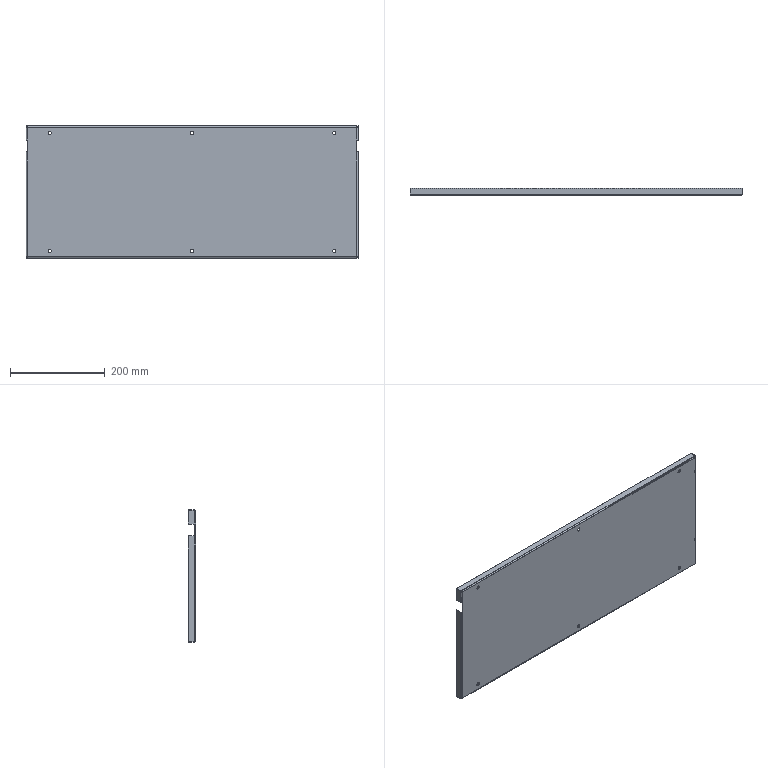Part | STEP file | 1 solid | 82 faces | box 700 x 15 x 279 mm | volume 263308 mm3 | plane 58 | cylinder 24 | commonest cylinder face diameters 7 x12 3 x6 5.4 x6